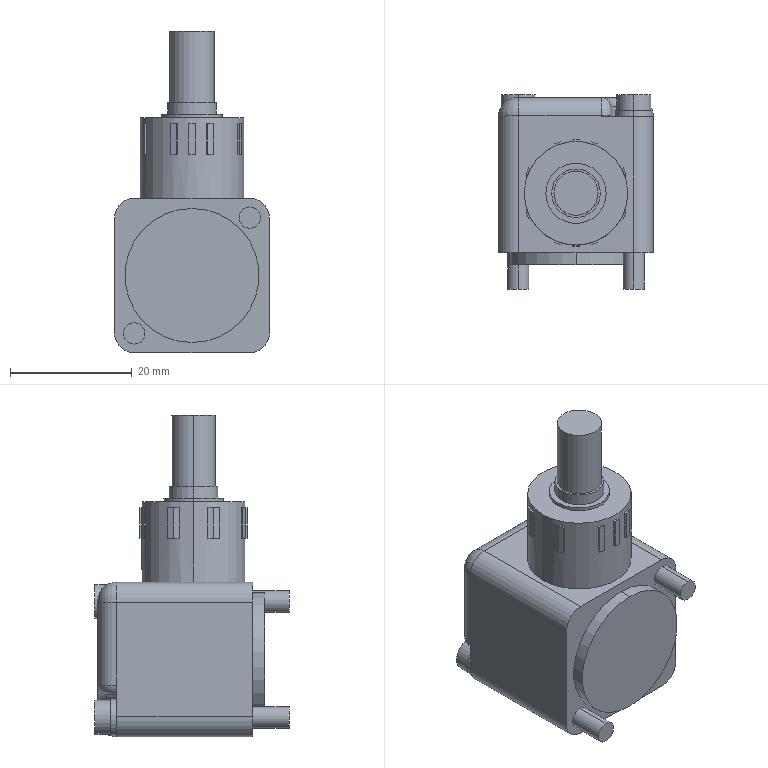Part | SolidWorks | features BaseBody 1 | 1 solid | 121 faces | box 25.4 x 31.9 x 52.8 mm | volume 20430 mm3 | plane 73 | cylinder 40 | torus 8 | commonest cylinder face diameters 3 x8 6 x8 3.5 x4 5.6 x4 6.6 x4 7.25 x2